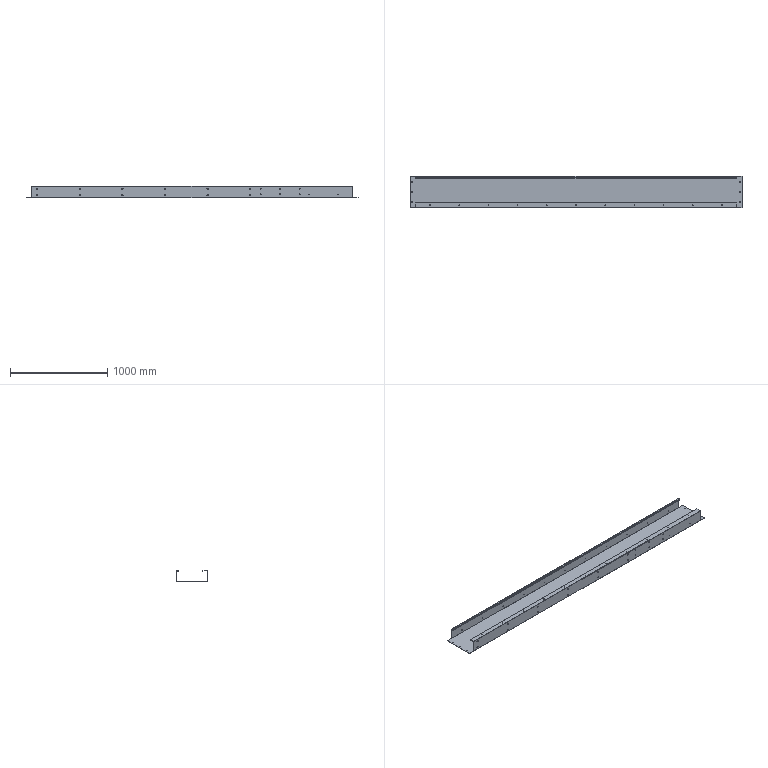Part | STEP file | SX-002-01 | 1 solid | 215 faces | box 3411 x 320 x 122 mm | volume 4301927 mm3 | cylinder 132 | plane 83 | commonest cylinder face diameters 5.4 x70 10 x24 7 x12 10.5 x12 0.4 x6 4.4 x6